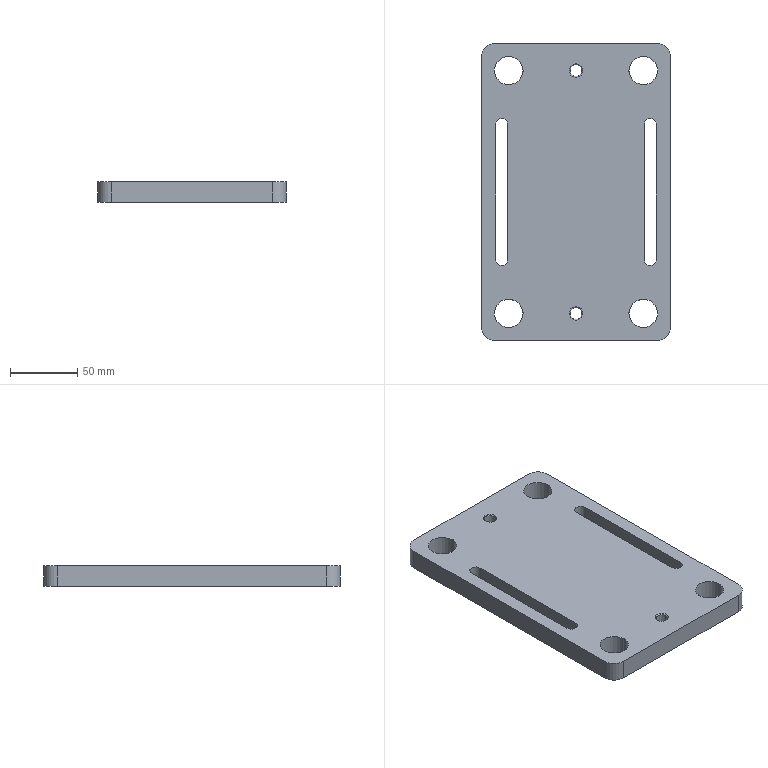Part | STEP file | YBQDJ-YL-4 | 1 solid | 88 faces | box 140 x 220 x 15 mm | volume 408740 mm3 | cylinder 42 | cone 36 | plane 10 | commonest cylinder face diameters 2.5 x16 4 x8 1 x4 9 x4 20 x4 21.01 x4